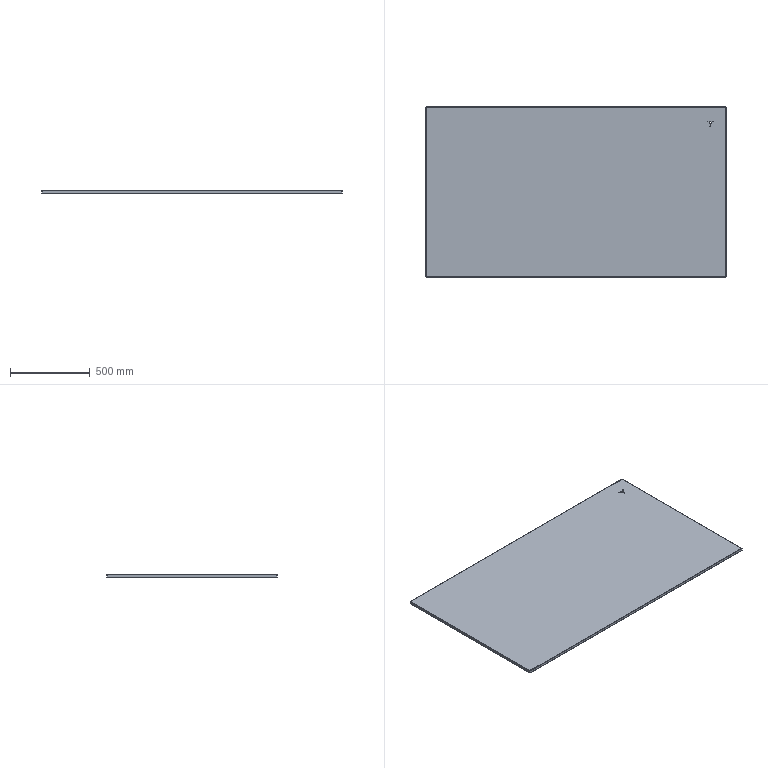Part | SolidWorks | features EdgeFlange 2, HoleWzd 2, CirPattern 1, FlatPattern 1, SMBaseFlange 1, SheetMetal 1 | 1 solid | 78 faces | box 1886 x 1068 x 18.5 mm | volume 3323198 mm3 | plane 38 | cylinder 24 | spline 16 | commonest cylinder face diameters 1 x8 4 x8 3.3 x6 14 x2